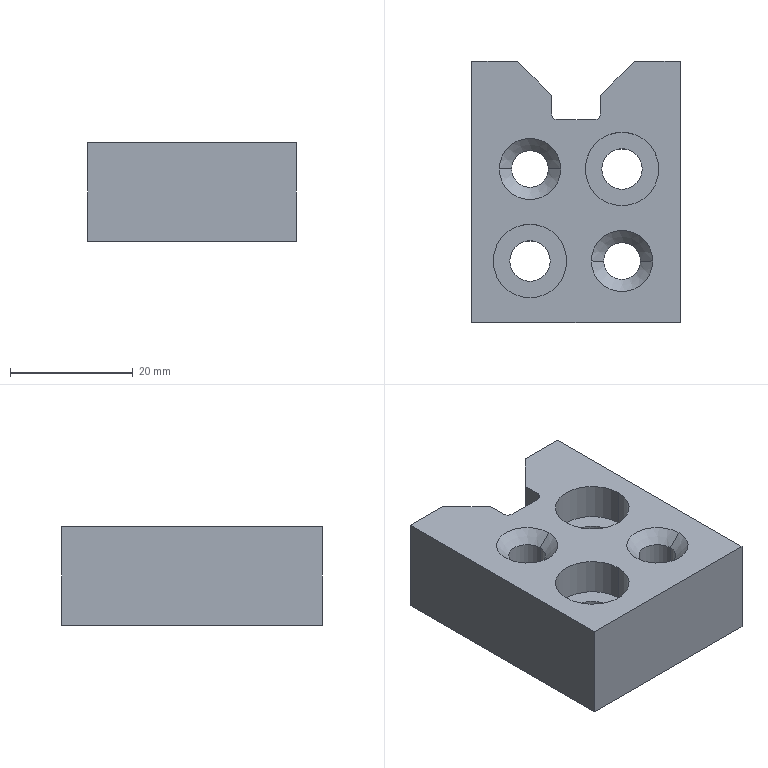Part | SolidWorks | features Chamfer 2, Cut 2, Fillet 2, HoleWzd 2, Extrusion 1, ICE 1 | 1 solid | 36 faces | box 34 x 42.517 x 16 mm | volume 18300 mm3 | cylinder 14 | plane 14 | cone 8 | commonest cylinder face diameters 6 x4 6.6 x4 12 x4 2 x2
STEP:
#1=CARTESIAN_POINT('',(-10.8,15.849,0.));
#2=VERTEX_POINT('',#1);
#3=CARTESIAN_POINT('',(-4.2,15.849,0.));
#4=VERTEX_POINT('',#3);
#5=CARTESIAN_POINT('',(-7.5,15.849,0.));
#6=DIRECTION('',(0.,0.,1.));
#7=DIRECTION('',(1.,0.,0.));
#8=AXIS2_PLACEMENT_3D('',#5,#6,#7);
#9=CIRCLE('',#8,3.3);
#10=EDGE_CURVE('',#2,#4,#9,.T.);
#11=ORIENTED_EDGE('',*,*,#10,.F.);
#12=CARTESIAN_POINT('',(-10.8,15.849,10.));
#13=VERTEX_POINT('',#12);
#14=CARTESIAN_POINT('',(-10.8,15.849,16.));
#15=DIRECTION('',(0.,0.,1.));
#16=VECTOR('',#15,1000.);
#17=LINE('',#14,#16);
#18=EDGE_CURVE('',#2,#13,#17,.T.);
#19=ORIENTED_EDGE('',*,*,#18,.T.);
#20=CARTESIAN_POINT('',(-4.2,15.849,10.));
#21=VERTEX_POINT('',#20);
#22=CARTESIAN_POINT('',(-7.5,15.849,10.));
#23=DIRECTION('',(0.,0.,1.));
#24=DIRECTION('',(1.,0.,0.));
#25=AXIS2_PLACEMENT_3D('',#22,#23,#24);
#26=CIRCLE('',#25,3.3);
#27=EDGE_CURVE('',#13,#21,#26,.T.);
#28=ORIENTED_EDGE('',*,*,#27,.T.);
#29=CARTESIAN_POINT('',(-4.2,15.849,16.));
#30=DIRECTION('',(0.,0.,1.));
#31=VECTOR('',#30,1000.);
#32=LINE('',#29,#31);
#33=EDGE_CURVE('',#4,#21,#32,.T.);
#34=ORIENTED_EDGE('',*,*,#33,.F.);
#35=EDGE_LOOP('',(#11,#19,#28,#34));
#36=FACE_OUTER_BOUND('',#35,.T.);
#37=CARTESIAN_POINT('',(-7.5,15.849,16.));
#38=DIRECTION('',(0.,0.,1.));
#39=DIRECTION('',(1.,0.,0.));
#40=AXIS2_PLACEMENT_3D('',#37,#38,#39);
#41=CYLINDRICAL_SURFACE('',#40,3.3);
#42=ADVANCED_FACE('',(#36),#41,.F.);
#43=CARTESIAN_POINT('',(-13.5,15.849,10.));
#44=VERTEX_POINT('',#43);
#45=CARTESIAN_POINT('',(-1.5,15.849,10.));
#46=VERTEX_POINT('',#45);
#47=CARTESIAN_POINT('',(-7.5,15.849,10.));
#48=DIRECTION('',(0.,0.,1.));
#49=DIRECTION('',(1.,0.,0.));
#50=AXIS2_PLACEMENT_3D('',#47,#48,#49);
#51=CIRCLE('',#50,6.);
#52=EDGE_CURVE('',#44,#46,#51,.T.);
#53=ORIENTED_EDGE('',*,*,#52,.F.);
#54=CARTESIAN_POINT('',(-13.5,15.849,16.));
#55=VERTEX_POINT('',#54);
#56=CARTESIAN_POINT('',(-13.5,15.849,16.));
#57=DIRECTION('',(0.,0.,1.));
#58=VECTOR('',#57,1000.);
#59=LINE('',#56,#58);
#60=EDGE_CURVE('',#44,#55,#59,.T.);
#61=ORIENTED_EDGE('',*,*,#60,.T.);
#62=CARTESIAN_POINT('',(-1.5,15.849,16.));
#63=VERTEX_POINT('',#62);
#64=CARTESIAN_POINT('',(-7.5,15.849,16.));
#65=DIRECTION('',(0.,0.,1.));
#66=DIRECTION('',(1.,0.,0.));
#67=AXIS2_PLACEMENT_3D('',#64,#65,#66);
#68=CIRCLE('',#67,6.);
#69=EDGE_CURVE('',#55,#63,#68,.T.);
#70=ORIENTED_EDGE('',*,*,#69,.T.);
#71=CARTESIAN_POINT('',(-1.5,15.849,16.));
#72=DIRECTION('',(0.,0.,1.));
#73=VECTOR('',#72,1000.);
#74=LINE('',#71,#73);
#75=EDGE_CURVE('',#46,#63,#74,.T.);
#76=ORIENTED_EDGE('',*,*,#75,.F.);
#77=EDGE_LOOP('',(#53,#61,#70,#76));
#78=FACE_OUTER_BOUND('',#77,.T.);
#79=CARTESIAN_POINT('',(-7.5,15.849,16.));
#80=DIRECTION('',(0.,0.,1.));
#81=DIRECTION('',(1.,0.,0.));
#82=AXIS2_PLACEMENT_3D('',#79,#80,#81);
#83=CYLINDRICAL_SURFACE('',#82,6.);
#84=ADVANCED_FACE('',(#78),#83,.F.);
#85=CARTESIAN_POINT('',(10.5,15.849,2.));
#86=VERTEX_POINT('',#85);
#87=CARTESIAN_POINT('',(4.5,15.849,2.));
#88=VERTEX_POINT('',#87);
#89=CARTESIAN_POINT('',(7.5,15.849,2.));
#90=DIRECTION('',(0.,0.,-1.));
#91=DIRECTION('',(1.,0.,0.));
#92=AXIS2_PLACEMENT_3D('',#89,#90,#91);
#93=CIRCLE('',#92,3.);
#94=EDGE_CURVE('',#86,#88,#93,.T.);
#95=ORIENTED_EDGE('',*,*,#94,.F.);
#96=CARTESIAN_POINT('',(12.5,15.849,0.));
#97=VERTEX_POINT('',#96);
#98=CARTESIAN_POINT('',(12.5,15.849,0.));
#99=DIRECTION('',(0.7071,0.,-0.7071));
#100=VECTOR('',#99,1000.);
#101=LINE('',#98,#100);
#102=EDGE_CURVE('',#86,#97,#101,.T.);
#103=ORIENTED_EDGE('',*,*,#102,.T.);
#104=CARTESIAN_POINT('',(2.5,15.849,0.));
#105=VERTEX_POINT('',#104);
#106=CARTESIAN_POINT('',(7.5,15.849,0.));
#107=DIRECTION('',(0.,0.,1.));
#108=DIRECTION('',(1.,0.,0.));
#109=AXIS2_PLACEMENT_3D('',#106,#107,#108);
#110=CIRCLE('',#109,5.);
#111=EDGE_CURVE('',#105,#97,#110,.T.);
#112=ORIENTED_EDGE('',*,*,#111,.F.);
#113=CARTESIAN_POINT('',(2.5,15.849,0.));
#114=DIRECTION('',(-0.7071,0.,-0.7071));
#115=VECTOR('',#114,1000.);
#116=LINE('',#113,#115);
#117=EDGE_CURVE('',#88,#105,#116,.T.);
#118=ORIENTED_EDGE('',*,*,#117,.F.);
#119=EDGE_LOOP('',(#95,#103,#112,#118));
#120=FACE_OUTER_BOUND('',#119,.T.);
#121=CARTESIAN_POINT('',(7.5,15.849,0.));
#122=DIRECTION('',(0.,0.,-1.));
#123=DIRECTION('',(-1.,0.,0.));
#124=AXIS2_PLACEMENT_3D('',#121,#122,#123);
#125=CONICAL_SURFACE('',#124,5.,0.7854);
#126=ADVANCED_FACE('',(#120),#125,.F.);
#127=CARTESIAN_POINT('',(-4.5,30.849,2.));
#128=VERTEX_POINT('',#127);
#129=CARTESIAN_POINT('',(-10.5,30.849,2.));
#130=VERTEX_POINT('',#129);
#131=CARTESIAN_POINT('',(-7.5,30.849,2.));
#132=DIRECTION('',(0.,0.,-1.));
#133=DIRECTION('',(1.,0.,0.));
#134=AXIS2_PLACEMENT_3D('',#131,#132,#133);
#135=CIRCLE('',#134,3.);
#136=EDGE_CURVE('',#128,#130,#135,.T.);
#137=ORIENTED_EDGE('',*,*,#136,.F.);
#138=CARTESIAN_POINT('',(-2.5,30.849,0.));
#139=VERTEX_POINT('',#138);
#140=CARTESIAN_POINT('',(-2.5,30.849,0.));
#141=DIRECTION('',(0.7071,0.,-0.7071));
#142=VECTOR('',#141,1000.);
#143=LINE('',#140,#142);
#144=EDGE_CURVE('',#128,#139,#143,.T.);
#145=ORIENTED_EDGE('',*,*,#144,.T.);
#146=CARTESIAN_POINT('',(-12.5,30.849,0.));
#147=VERTEX_POINT('',#146);
#148=CARTESIAN_POINT('',(-7.5,30.849,0.));
#149=DIRECTION('',(0.,0.,1.));
#150=DIRECTION('',(1.,0.,0.));
#151=AXIS2_PLACEMENT_3D('',#148,#149,#150);
#152=CIRCLE('',#151,5.);
#153=EDGE_CURVE('',#147,#139,#152,.T.);
#154=ORIENTED_EDGE('',*,*,#153,.F.);
#155=CARTESIAN_POINT('',(-12.5,30.849,0.));
#156=DIRECTION('',(-0.7071,0.,-0.7071));
#157=VECTOR('',#156,1000.);
#158=LINE('',#155,#157);
#159=EDGE_CURVE('',#130,#147,#158,.T.);
#160=ORIENTED_EDGE('',*,*,#159,.F.);
#161=EDGE_LOOP('',(#137,#145,#154,#160));
#162=FACE_OUTER_BOUND('',#161,.T.);
#163=CARTESIAN_POINT('',(-7.5,30.849,0.));
#164=DIRECTION('',(0.,0.,-1.));
#165=DIRECTION('',(-1.,0.,0.));
#166=AXIS2_PLACEMENT_3D('',#163,#164,#165);
#167=CONICAL_SURFACE('',#166,5.,0.7854);
#168=ADVANCED_FACE('',(#162),#167,.F.);
#169=CARTESIAN_POINT('',(4.5,15.849,14.));
#170=VERTEX_POINT('',#169);
#171=CARTESIAN_POINT('',(10.5,15.849,14.));
#172=VERTEX_POINT('',#171);
#173=CARTESIAN_POINT('',(7.5,15.849,14.));
#174=DIRECTION('',(0.,0.,1.));
#175=DIRECTION('',(1.,0.,0.));
#176=AXIS2_PLACEMENT_3D('',#173,#174,#175);
#177=CIRCLE('',#176,3.);
#178=EDGE_CURVE('',#170,#172,#177,.T.);
#179=ORIENTED_EDGE('',*,*,#178,.F.);
#180=CARTESIAN_POINT('',(2.5,15.849,16.));
#181=VERTEX_POINT('',#180);
#182=CARTESIAN_POINT('',(4.5,15.849,14.));
#183=DIRECTION('',(-0.7071,0.,0.7071));
#184=VECTOR('',#183,1000.);
#185=LINE('',#182,#184);
#186=EDGE_CURVE('',#170,#181,#185,.T.);
#187=ORIENTED_EDGE('',*,*,#186,.T.);
#188=CARTESIAN_POINT('',(12.5,15.849,16.));
#189=VERTEX_POINT('',#188);
#190=CARTESIAN_POINT('',(7.5,15.849,16.));
#191=DIRECTION('',(0.,0.,-1.));
#192=DIRECTION('',(1.,0.,0.));
#193=AXIS2_PLACEMENT_3D('',#190,#191,#192);
#194=CIRCLE('',#193,5.);
#195=EDGE_CURVE('',#189,#181,#194,.T.);
#196=ORIENTED_EDGE('',*,*,#195,.F.);
#197=CARTESIAN_POINT('',(10.5,15.849,14.));
#198=DIRECTION('',(0.7071,0.,0.7071));
#199=VECTOR('',#198,1000.);
#200=LINE('',#197,#199);
#201=EDGE_CURVE('',#172,#189,#200,.T.);
#202=ORIENTED_EDGE('',*,*,#201,.F.);
#203=EDGE_LOOP('',(#179,#187,#196,#202));
#204=FACE_OUTER_BOUND('',#203,.T.);
#205=CARTESIAN_POINT('',(7.5,15.849,14.));
#206=DIRECTION('',(0.,0.,1.));
#207=DIRECTION('',(1.,0.,0.));
#208=AXIS2_PLACEMENT_3D('',#205,#206,#207);
#209=CONICAL_SURFACE('',#208,3.,0.7854);
#210=ADVANCED_FACE('',(#204),#209,.F.);
#211=CARTESIAN_POINT('',(-10.5,30.849,14.));
#212=VERTEX_POINT('',#211);
#213=CARTESIAN_POINT('',(-4.5,30.849,14.));
#214=VERTEX_POINT('',#213);
#215=CARTESIAN_POINT('',(-7.5,30.849,14.));
#216=DIRECTION('',(0.,0.,1.));
#217=DIRECTION('',(1.,0.,0.));
#218=AXIS2_PLACEMENT_3D('',#215,#216,#217);
#219=CIRCLE('',#218,3.);
#220=EDGE_CURVE('',#212,#214,#219,.T.);
#221=ORIENTED_EDGE('',*,*,#220,.F.);
#222=CARTESIAN_POINT('',(-12.5,30.849,16.));
#223=VERTEX_POINT('',#222);
#224=CARTESIAN_POINT('',(-10.5,30.849,14.));
#225=DIRECTION('',(-0.7071,0.,0.7071));
#226=VECTOR('',#225,1000.);
#227=LINE('',#224,#226);
#228=EDGE_CURVE('',#212,#223,#227,.T.);
#229=ORIENTED_EDGE('',*,*,#228,.T.);
#230=CARTESIAN_POINT('',(-2.5,30.849,16.));
#231=VERTEX_POINT('',#230);
#232=CARTESIAN_POINT('',(-7.5,30.849,16.));
#233=DIRECTION('',(0.,0.,-1.));
#234=DIRECTION('',(1.,0.,0.));
#235=AXIS2_PLACEMENT_3D('',#232,#233,#234);
#236=CIRCLE('',#235,5.);
#237=EDGE_CURVE('',#231,#223,#236,.T.);
#238=ORIENTED_EDGE('',*,*,#237,.F.);
#239=CARTESIAN_POINT('',(-4.5,30.849,14.));
#240=DIRECTION('',(0.7071,0.,0.7071));
#241=VECTOR('',#240,1000.);
#242=LINE('',#239,#241);
#243=EDGE_CURVE('',#214,#231,#242,.T.);
#244=ORIENTED_EDGE('',*,*,#243,.F.);
#245=EDGE_LOOP('',(#221,#229,#238,#244));
#246=FACE_OUTER_BOUND('',#245,.T.);
#247=CARTESIAN_POINT('',(-7.5,30.849,14.));
#248=DIRECTION('',(0.,0.,1.));
#249=DIRECTION('',(1.,0.,0.));
#250=AXIS2_PLACEMENT_3D('',#247,#248,#249);
#251=CONICAL_SURFACE('',#250,3.,0.7854);
#252=ADVANCED_FACE('',(#246),#251,.F.);
#253=ORIENTED_EDGE('',*,*,#94,.T.);
#254=CARTESIAN_POINT('',(4.5,15.849,-9.));
#255=DIRECTION('',(0.,0.,1.));
#256=VECTOR('',#255,1000.);
#257=LINE('',#254,#256);
#258=EDGE_CURVE('',#88,#170,#257,.T.);
#259=ORIENTED_EDGE('',*,*,#258,.T.);
#260=ORIENTED_EDGE('',*,*,#178,.T.);
#261=CARTESIAN_POINT('',(10.5,15.849,-9.));
#262=DIRECTION('',(0.,0.,1.));
#263=VECTOR('',#262,1000.);
#264=LINE('',#261,#263);
#265=EDGE_CURVE('',#86,#172,#264,.T.);
#266=ORIENTED_EDGE('',*,*,#265,.F.);
#267=EDGE_LOOP('',(#253,#259,#260,#266));
#268=FACE_OUTER_BOUND('',#267,.T.);
#269=CARTESIAN_POINT('',(7.5,15.849,-9.));
#270=DIRECTION('',(0.,0.,1.));
#271=DIRECTION('',(1.,0.,0.));
#272=AXIS2_PLACEMENT_3D('',#269,#270,#271);
#273=CYLINDRICAL_SURFACE('',#272,3.);
#274=ADVANCED_FACE('',(#268),#273,.F.);
#275=ORIENTED_EDGE('',*,*,#136,.T.);
#276=CARTESIAN_POINT('',(-10.5,30.849,-9.));
#277=DIRECTION('',(0.,0.,1.));
#278=VECTOR('',#277,1000.);
#279=LINE('',#276,#278);
#280=EDGE_CURVE('',#130,#212,#279,.T.);
#281=ORIENTED_EDGE('',*,*,#280,.T.);
#282=ORIENTED_EDGE('',*,*,#220,.T.);
#283=CARTESIAN_POINT('',(-4.5,30.849,-9.));
#284=DIRECTION('',(0.,0.,1.));
#285=VECTOR('',#284,1000.);
#286=LINE('',#283,#285);
#287=EDGE_CURVE('',#128,#214,#286,.T.);
#288=ORIENTED_EDGE('',*,*,#287,.F.);
#289=EDGE_LOOP('',(#275,#281,#282,#288));
#290=FACE_OUTER_BOUND('',#289,.T.);
#291=CARTESIAN_POINT('',(-7.5,30.849,-9.));
#292=DIRECTION('',(0.,0.,1.));
#293=DIRECTION('',(1.,0.,0.));
#294=AXIS2_PLACEMENT_3D('',#291,#292,#293);
#295=CYLINDRICAL_SURFACE('',#294,3.);
#296=ADVANCED_FACE('',(#290),#295,.F.);
#297=CARTESIAN_POINT('',(4.2,30.849,0.));
#298=VERTEX_POINT('',#297);
#299=CARTESIAN_POINT('',(10.8,30.849,0.));
#300=VERTEX_POINT('',#299);
#301=CARTESIAN_POINT('',(7.5,30.849,0.));
#302=DIRECTION('',(0.,0.,1.));
#303=DIRECTION('',(1.,0.,0.));
#304=AXIS2_PLACEMENT_3D('',#301,#302,#303);
#305=CIRCLE('',#304,3.3);
#306=EDGE_CURVE('',#298,#300,#305,.T.);
#307=ORIENTED_EDGE('',*,*,#306,.F.);
#308=CARTESIAN_POINT('',(4.2,30.849,10.));
#309=VERTEX_POINT('',#308);
#310=CARTESIAN_POINT('',(4.2,30.849,16.));
#311=DIRECTION('',(0.,0.,1.));
#312=VECTOR('',#311,1000.);
#313=LINE('',#310,#312);
#314=EDGE_CURVE('',#298,#309,#313,.T.);
#315=ORIENTED_EDGE('',*,*,#314,.T.);
#316=CARTESIAN_POINT('',(10.8,30.849,10.));
#317=VERTEX_POINT('',#316);
#318=CARTESIAN_POINT('',(7.5,30.849,10.));
#319=DIRECTION('',(0.,0.,1.));
#320=DIRECTION('',(1.,0.,0.));
#321=AXIS2_PLACEMENT_3D('',#318,#319,#320);
#322=CIRCLE('',#321,3.3);
#323=EDGE_CURVE('',#309,#317,#322,.T.);
#324=ORIENTED_EDGE('',*,*,#323,.T.);
#325=CARTESIAN_POINT('',(10.8,30.849,16.));
#326=DIRECTION('',(0.,0.,1.));
#327=VECTOR('',#326,1000.);
#328=LINE('',#325,#327);
#329=EDGE_CURVE('',#300,#317,#328,.T.);
#330=ORIENTED_EDGE('',*,*,#329,.F.);
#331=EDGE_LOOP('',(#307,#315,#324,#330));
#332=FACE_OUTER_BOUND('',#331,.T.);
#333=CARTESIAN_POINT('',(7.5,30.849,16.));
#334=DIRECTION('',(0.,0.,1.));
#335=DIRECTION('',(1.,0.,0.));
#336=AXIS2_PLACEMENT_3D('',#333,#334,#335);
#337=CYLINDRICAL_SURFACE('',#336,3.3);
#338=ADVANCED_FACE('',(#332),#337,.F.);
#339=CARTESIAN_POINT('',(1.5,30.849,10.));
#340=VERTEX_POINT('',#339);
#341=CARTESIAN_POINT('',(13.5,30.849,10.));
#342=VERTEX_POINT('',#341);
#343=CARTESIAN_POINT('',(7.5,30.849,10.));
#344=DIRECTION('',(0.,0.,1.));
#345=DIRECTION('',(1.,0.,0.));
#346=AXIS2_PLACEMENT_3D('',#343,#344,#345);
#347=CIRCLE('',#346,6.);
#348=EDGE_CURVE('',#340,#342,#347,.T.);
#349=ORIENTED_EDGE('',*,*,#348,.F.);
#350=CARTESIAN_POINT('',(1.5,30.849,16.));
#351=VERTEX_POINT('',#350);
#352=CARTESIAN_POINT('',(1.5,30.849,16.));
#353=DIRECTION('',(0.,0.,1.));
#354=VECTOR('',#353,1000.);
#355=LINE('',#352,#354);
#356=EDGE_CURVE('',#340,#351,#355,.T.);
#357=ORIENTED_EDGE('',*,*,#356,.T.);
#358=CARTESIAN_POINT('',(13.5,30.849,16.));
#359=VERTEX_POINT('',#358);
#360=CARTESIAN_POINT('',(7.5,30.849,16.));
#361=DIRECTION('',(0.,0.,1.));
#362=DIRECTION('',(1.,0.,0.));
#363=AXIS2_PLACEMENT_3D('',#360,#361,#362);
#364=CIRCLE('',#363,6.);
#365=EDGE_CURVE('',#351,#359,#364,.T.);
#366=ORIENTED_EDGE('',*,*,#365,.T.);
#367=CARTESIAN_POINT('',(13.5,30.849,16.));
#368=DIRECTION('',(0.,0.,1.));
#369=VECTOR('',#368,1000.);
#370=LINE('',#367,#369);
#371=EDGE_CURVE('',#342,#359,#370,.T.);
#372=ORIENTED_EDGE('',*,*,#371,.F.);
#373=EDGE_LOOP('',(#349,#357,#366,#372));
#374=FACE_OUTER_BOUND('',#373,.T.);
#375=CARTESIAN_POINT('',(7.5,30.849,16.));
#376=DIRECTION('',(0.,0.,1.));
#377=DIRECTION('',(1.,0.,0.));
#378=AXIS2_PLACEMENT_3D('',#375,#376,#377);
#379=CYLINDRICAL_SURFACE('',#378,6.);
#380=ADVANCED_FACE('',(#374),#379,.F.);
#381=CARTESIAN_POINT('',(-17.,48.365,16.));
#382=VERTEX_POINT('',#381);
#383=CARTESIAN_POINT('',(-17.,5.849,16.));
#384=VERTEX_POINT('',#383);
#385=CARTESIAN_POINT('',(-17.,50.849,16.));
#386=DIRECTION('',(0.,-1.,0.));
#387=VECTOR('',#386,1000.);
#388=LINE('',#385,#387);
#389=EDGE_CURVE('',#382,#384,#388,.T.);
#390=ORIENTED_EDGE('',*,*,#389,.F.);
#391=CARTESIAN_POINT('',(-17.,48.365,0.));
#392=VERTEX_POINT('',#391);
#393=CARTESIAN_POINT('',(-17.,48.365,16.));
#394=DIRECTION('',(0.,0.,-1.));
#395=VECTOR('',#394,1000.);
#396=LINE('',#393,#395);
#397=EDGE_CURVE('',#382,#392,#396,.T.);
#398=ORIENTED_EDGE('',*,*,#397,.T.);
#399=CARTESIAN_POINT('',(-17.,5.849,0.));
#400=VERTEX_POINT('',#399);
#401=CARTESIAN_POINT('',(-17.,50.849,0.));
#402=DIRECTION('',(0.,-1.,0.));
#403=VECTOR('',#402,1000.);
#404=LINE('',#401,#403);
#405=EDGE_CURVE('',#392,#400,#404,.T.);
#406=ORIENTED_EDGE('',*,*,#405,.T.);
#407=CARTESIAN_POINT('',(-17.,5.849,16.));
#408=DIRECTION('',(0.,0.,-1.));
#409=VECTOR('',#408,1000.);
#410=LINE('',#407,#409);
#411=EDGE_CURVE('',#384,#400,#410,.T.);
#412=ORIENTED_EDGE('',*,*,#411,.F.);
#413=EDGE_LOOP('',(#390,#398,#406,#412));
#414=FACE_OUTER_BOUND('',#413,.T.);
#415=CARTESIAN_POINT('',(-17.,50.849,16.));
#416=DIRECTION('',(1.,0.,0.));
#417=DIRECTION('',(0.,1.,0.));
#418=AXIS2_PLACEMENT_3D('',#415,#416,#417);
#419=PLANE('',#418);
#420=ADVANCED_FACE('',(#414),#419,.F.);
#421=CARTESIAN_POINT('',(17.,5.849,0.));
#422=VERTEX_POINT('',#421);
#423=CARTESIAN_POINT('',(-17.,5.849,0.));
#424=DIRECTION('',(1.,0.,0.));
#425=VECTOR('',#424,1000.);
#426=LINE('',#423,#425);
#427=EDGE_CURVE('',#400,#422,#426,.T.);
#428=ORIENTED_EDGE('',*,*,#427,.T.);
#429=CARTESIAN_POINT('',(17.,5.849,16.));
#430=VERTEX_POINT('',#429);
#431=CARTESIAN_POINT('',(17.,5.849,16.));
#432=DIRECTION('',(0.,0.,-1.));
#433=VECTOR('',#432,1000.);
#434=LINE('',#431,#433);
#435=EDGE_CURVE('',#430,#422,#434,.T.);
#436=ORIENTED_EDGE('',*,*,#435,.F.);
#437=CARTESIAN_POINT('',(-17.,5.849,16.));
#438=DIRECTION('',(1.,0.,0.));
#439=VECTOR('',#438,1000.);
#440=LINE('',#437,#439);
#441=EDGE_CURVE('',#384,#430,#440,.T.);
#442=ORIENTED_EDGE('',*,*,#441,.F.);
#443=ORIENTED_EDGE('',*,*,#411,.T.);
#444=EDGE_LOOP('',(#428,#436,#442,#443));
#445=FACE_OUTER_BOUND('',#444,.T.);
#446=CARTESIAN_POINT('',(-17.,5.849,16.));
#447=DIRECTION('',(0.,1.,0.));
#448=DIRECTION('',(-1.,0.,0.));
#449=AXIS2_PLACEMENT_3D('',#446,#447,#448);
#450=PLANE('',#449);
#451=ADVANCED_FACE('',(#445),#450,.F.);
#452=CARTESIAN_POINT('',(17.,48.365,0.));
#453=VERTEX_POINT('',#452);
#454=CARTESIAN_POINT('',(17.,50.849,0.));
#455=DIRECTION('',(0.,1.,0.));
#456=VECTOR('',#455,1000.);
#457=LINE('',#454,#456);
#458=EDGE_CURVE('',#422,#453,#457,.T.);
#459=ORIENTED_EDGE('',*,*,#458,.T.);
#460=CARTESIAN_POINT('',(17.,48.365,16.));
#461=VERTEX_POINT('',#460);
#462=CARTESIAN_POINT('',(17.,48.365,16.));
#463=DIRECTION('',(0.,0.,1.));
#464=VECTOR('',#463,1000.);
#465=LINE('',#462,#464);
#466=EDGE_CURVE('',#453,#461,#465,.T.);
#467=ORIENTED_EDGE('',*,*,#466,.T.);
#468=CARTESIAN_POINT('',(17.,50.849,16.));
#469=DIRECTION('',(0.,1.,0.));
#470=VECTOR('',#469,1000.);
#471=LINE('',#468,#470);
#472=EDGE_CURVE('',#430,#461,#471,.T.);
#473=ORIENTED_EDGE('',*,*,#472,.F.);
#474=ORIENTED_EDGE('',*,*,#435,.T.);
#475=EDGE_LOOP('',(#459,#467,#473,#474));
#476=FACE_OUTER_BOUND('',#475,.T.);
#477=CARTESIAN_POINT('',(17.,50.849,16.));
#478=DIRECTION('',(-1.,0.,0.));
#479=DIRECTION('',(0.,-1.,0.));
#480=AXIS2_PLACEMENT_3D('',#477,#478,#479);
#481=PLANE('',#480);
#482=ADVANCED_FACE('',(#476),#481,.F.);
#483=CARTESIAN_POINT('',(-9.517,48.365,16.));
#484=VERTEX_POINT('',#483);
#485=CARTESIAN_POINT('',(-19.125,48.365,16.));
#486=DIRECTION('',(1.,0.,0.));
#487=VECTOR('',#486,1000.);
#488=LINE('',#485,#487);
#489=EDGE_CURVE('',#382,#484,#488,.T.);
#490=ORIENTED_EDGE('',*,*,#489,.F.);
#491=ORIENTED_EDGE('',*,*,#389,.T.);
#492=ORIENTED_EDGE('',*,*,#441,.T.);
#493=ORIENTED_EDGE('',*,*,#472,.T.);
#494=CARTESIAN_POINT('',(9.517,48.365,16.));
#495=VERTEX_POINT('',#494);
#496=CARTESIAN_POINT('',(-19.125,48.365,16.));
#497=DIRECTION('',(1.,0.,0.));
#498=VECTOR('',#497,1000.);
#499=LINE('',#496,#498);
#500=EDGE_CURVE('',#495,#461,#499,.T.);
#501=ORIENTED_EDGE('',*,*,#500,.F.);
#502=CARTESIAN_POINT('',(4.,42.849,16.));
#503=VERTEX_POINT('',#502);
#504=CARTESIAN_POINT('',(12.,50.849,16.));
#505=DIRECTION('',(0.7071,0.7071,0.));
#506=VECTOR('',#505,1000.);
#507=LINE('',#504,#506);
#508=EDGE_CURVE('',#503,#495,#507,.T.);
#509=ORIENTED_EDGE('',*,*,#508,.F.);
#510=CARTESIAN_POINT('',(4.,39.849,16.));
#511=VERTEX_POINT('',#510);
#512=CARTESIAN_POINT('',(4.,38.849,16.));
#513=DIRECTION('',(0.,1.,0.));
#514=VECTOR('',#513,1000.);
#515=LINE('',#512,#514);
#516=EDGE_CURVE('',#511,#503,#515,.T.);
#517=ORIENTED_EDGE('',*,*,#516,.F.);
#518=CARTESIAN_POINT('',(3.,38.849,16.));
#519=VERTEX_POINT('',#518);
#520=CARTESIAN_POINT('',(3.,39.849,16.));
#521=DIRECTION('',(0.,0.,-1.));
#522=DIRECTION('',(1.,0.,0.));
#523=AXIS2_PLACEMENT_3D('',#520,#521,#522);
#524=CIRCLE('',#523,1.);
#525=EDGE_CURVE('',#511,#519,#524,.T.);
#526=ORIENTED_EDGE('',*,*,#525,.T.);
#527=CARTESIAN_POINT('',(-3.,38.849,16.));
#528=VERTEX_POINT('',#527);
#529=CARTESIAN_POINT('',(-4.,38.849,16.));
#530=DIRECTION('',(1.,0.,0.));
#531=VECTOR('',#530,1000.);
#532=LINE('',#529,#531);
#533=EDGE_CURVE('',#528,#519,#532,.T.);
#534=ORIENTED_EDGE('',*,*,#533,.F.);
#535=CARTESIAN_POINT('',(-4.,39.849,16.));
#536=VERTEX_POINT('',#535);
#537=CARTESIAN_POINT('',(-3.,39.849,16.));
#538=DIRECTION('',(0.,0.,-1.));
#539=DIRECTION('',(1.,0.,0.));
#540=AXIS2_PLACEMENT_3D('',#537,#538,#539);
#541=CIRCLE('',#540,1.);
#542=EDGE_CURVE('',#528,#536,#541,.T.);
#543=ORIENTED_EDGE('',*,*,#542,.T.);
#544=CARTESIAN_POINT('',(-4.,42.849,16.));
#545=VERTEX_POINT('',#544);
#546=CARTESIAN_POINT('',(-4.,38.849,16.));
#547=DIRECTION('',(0.,-1.,0.));
#548=VECTOR('',#547,1000.);
#549=LINE('',#546,#548);
#550=EDGE_CURVE('',#545,#536,#549,.T.);
#551=ORIENTED_EDGE('',*,*,#550,.F.);
#552=CARTESIAN_POINT('',(-12.,50.849,16.));
#553=DIRECTION('',(0.7071,-0.7071,0.));
#554=VECTOR('',#553,1000.);
#555=LINE('',#552,#554);
#556=EDGE_CURVE('',#484,#545,#555,.T.);
#557=ORIENTED_EDGE('',*,*,#556,.F.);
#558=EDGE_LOOP('',(#490,#491,#492,#493,#501,#509,#517,#526,#534,#543,#551,#557));
#559=FACE_OUTER_BOUND('',#558,.T.);
#560=CARTESIAN_POINT('',(-7.5,15.849,16.));
#561=DIRECTION('',(0.,0.,1.));
#562=DIRECTION('',(1.,0.,0.));
#563=AXIS2_PLACEMENT_3D('',#560,#561,#562);
#564=CIRCLE('',#563,6.);
#565=EDGE_CURVE('',#63,#55,#564,.T.);
#566=ORIENTED_EDGE('',*,*,#565,.F.);
#567=ORIENTED_EDGE('',*,*,#69,.F.);
#568=EDGE_LOOP('',(#566,#567));
#569=FACE_BOUND('',#568,.T.);
#570=ORIENTED_EDGE('',*,*,#237,.T.);
#571=CARTESIAN_POINT('',(-7.5,30.849,16.));
#572=DIRECTION('',(0.,0.,-1.));
#573=DIRECTION('',(1.,0.,0.));
#574=AXIS2_PLACEMENT_3D('',#571,#572,#573);
#575=CIRCLE('',#574,5.);
#576=EDGE_CURVE('',#223,#231,#575,.T.);
#577=ORIENTED_EDGE('',*,*,#576,.T.);
#578=EDGE_LOOP('',(#570,#577));
#579=FACE_BOUND('',#578,.T.);
#580=ORIENTED_EDGE('',*,*,#195,.T.);
#581=CARTESIAN_POINT('',(7.5,15.849,16.));
#582=DIRECTION('',(0.,0.,-1.));
#583=DIRECTION('',(1.,0.,0.));
#584=AXIS2_PLACEMENT_3D('',#581,#582,#583);
#585=CIRCLE('',#584,5.);
#586=EDGE_CURVE('',#181,#189,#585,.T.);
#587=ORIENTED_EDGE('',*,*,#586,.T.);
#588=EDGE_LOOP('',(#580,#587));
#589=FACE_BOUND('',#588,.T.);
#590=CARTESIAN_POINT('',(7.5,30.849,16.));
#591=DIRECTION('',(0.,0.,1.));
#592=DIRECTION('',(1.,0.,0.));
#593=AXIS2_PLACEMENT_3D('',#590,#591,#592);
#594=CIRCLE('',#593,6.);
#595=EDGE_CURVE('',#359,#351,#594,.T.);
#596=ORIENTED_EDGE('',*,*,#595,.F.);
#597=ORIENTED_EDGE('',*,*,#365,.F.);
#598=EDGE_LOOP('',(#596,#597));
#599=FACE_BOUND('',#598,.T.);
#600=CARTESIAN_POINT('',(-17.,5.849,16.));
#601=DIRECTION('',(0.,0.,1.));
#602=DIRECTION('',(1.,0.,0.));
#603=AXIS2_PLACEMENT_3D('',#600,#601,#602);
#604=PLANE('',#603);
#605=ADVANCED_FACE('',(#559,#569,#579,#589,#599),#604,.T.);
#606=CARTESIAN_POINT('',(-7.5,15.849,0.));
#607=DIRECTION('',(0.,0.,1.));
#608=DIRECTION('',(1.,0.,0.));
#609=AXIS2_PLACEMENT_3D('',#606,#607,#608);
#610=CIRCLE('',#609,3.3);
#611=EDGE_CURVE('',#4,#2,#610,.T.);
#612=ORIENTED_EDGE('',*,*,#611,.T.);
#613=ORIENTED_EDGE('',*,*,#10,.T.);
#614=EDGE_LOOP('',(#612,#613));
#615=FACE_BOUND('',#614,.T.);
#616=ORIENTED_EDGE('',*,*,#153,.T.);
#617=CARTESIAN_POINT('',(-7.5,30.849,0.));
#618=DIRECTION('',(0.,0.,1.));
#619=DIRECTION('',(1.,0.,0.));
#620=AXIS2_PLACEMENT_3D('',#617,#618,#619);
#621=CIRCLE('',#620,5.);
#622=EDGE_CURVE('',#139,#147,#621,.T.);
#623=ORIENTED_EDGE('',*,*,#622,.T.);
#624=EDGE_LOOP('',(#616,#623));
#625=FACE_BOUND('',#624,.T.);
#626=ORIENTED_EDGE('',*,*,#111,.T.);
#627=CARTESIAN_POINT('',(7.5,15.849,0.));
#628=DIRECTION('',(0.,0.,1.));
#629=DIRECTION('',(1.,0.,0.));
#630=AXIS2_PLACEMENT_3D('',#627,#628,#629);
#631=CIRCLE('',#630,5.);
#632=EDGE_CURVE('',#97,#105,#631,.T.);
#633=ORIENTED_EDGE('',*,*,#632,.T.);
#634=EDGE_LOOP('',(#626,#633));
#635=FACE_BOUND('',#634,.T.);
#636=CARTESIAN_POINT('',(7.5,30.849,0.));
#637=DIRECTION('',(0.,0.,1.));
#638=DIRECTION('',(1.,0.,0.));
#639=AXIS2_PLACEMENT_3D('',#636,#637,#638);
#640=CIRCLE('',#639,3.3);
#641=EDGE_CURVE('',#300,#298,#640,.T.);
#642=ORIENTED_EDGE('',*,*,#641,.T.);
#643=ORIENTED_EDGE('',*,*,#306,.T.);
#644=EDGE_LOOP('',(#642,#643));
#645=FACE_BOUND('',#644,.T.);
#646=ORIENTED_EDGE('',*,*,#405,.F.);
#647=CARTESIAN_POINT('',(-9.517,48.365,0.));
#648=VERTEX_POINT('',#647);
#649=CARTESIAN_POINT('',(-19.125,48.365,0.));
#650=DIRECTION('',(1.,0.,0.));
#651=VECTOR('',#650,1000.);
#652=LINE('',#649,#651);
#653=EDGE_CURVE('',#392,#648,#652,.T.);
#654=ORIENTED_EDGE('',*,*,#653,.T.);
#655=CARTESIAN_POINT('',(-4.,42.849,0.));
#656=VERTEX_POINT('',#655);
#657=CARTESIAN_POINT('',(-12.,50.849,0.));
#658=DIRECTION('',(0.7071,-0.7071,0.));
#659=VECTOR('',#658,1000.);
#660=LINE('',#657,#659);
#661=EDGE_CURVE('',#648,#656,#660,.T.);
#662=ORIENTED_EDGE('',*,*,#661,.T.);
#663=CARTESIAN_POINT('',(-4.,39.849,0.));
#664=VERTEX_POINT('',#663);
#665=CARTESIAN_POINT('',(-4.,38.849,0.));
#666=DIRECTION('',(0.,-1.,0.));
#667=VECTOR('',#666,1000.);
#668=LINE('',#665,#667);
#669=EDGE_CURVE('',#656,#664,#668,.T.);
#670=ORIENTED_EDGE('',*,*,#669,.T.);
#671=CARTESIAN_POINT('',(-3.,38.849,0.));
#672=VERTEX_POINT('',#671);
#673=CARTESIAN_POINT('',(-3.,39.849,0.));
#674=DIRECTION('',(0.,0.,1.));
#675=DIRECTION('',(1.,0.,0.));
#676=AXIS2_PLACEMENT_3D('',#673,#674,#675);
#677=CIRCLE('',#676,1.);
#678=EDGE_CURVE('',#664,#672,#677,.T.);
#679=ORIENTED_EDGE('',*,*,#678,.T.);
#680=CARTESIAN_POINT('',(3.,38.849,0.));
#681=VERTEX_POINT('',#680);
#682=CARTESIAN_POINT('',(-4.,38.849,0.));
#683=DIRECTION('',(1.,0.,0.));
#684=VECTOR('',#683,1000.);
#685=LINE('',#682,#684);
#686=EDGE_CURVE('',#672,#681,#685,.T.);
#687=ORIENTED_EDGE('',*,*,#686,.T.);
#688=CARTESIAN_POINT('',(4.,39.849,0.));
#689=VERTEX_POINT('',#688);
#690=CARTESIAN_POINT('',(3.,39.849,0.));
#691=DIRECTION('',(0.,0.,1.));
#692=DIRECTION('',(1.,0.,0.));
#693=AXIS2_PLACEMENT_3D('',#690,#691,#692);
#694=CIRCLE('',#693,1.);
#695=EDGE_CURVE('',#681,#689,#694,.T.);
#696=ORIENTED_EDGE('',*,*,#695,.T.);
#697=CARTESIAN_POINT('',(4.,42.849,0.));
#698=VERTEX_POINT('',#697);
#699=CARTESIAN_POINT('',(4.,38.849,0.));
#700=DIRECTION('',(0.,1.,0.));
#701=VECTOR('',#700,1000.);
#702=LINE('',#699,#701);
#703=EDGE_CURVE('',#689,#698,#702,.T.);
#704=ORIENTED_EDGE('',*,*,#703,.T.);
#705=CARTESIAN_POINT('',(9.517,48.365,0.));
#706=VERTEX_POINT('',#705);
#707=CARTESIAN_POINT('',(12.,50.849,0.));
#708=DIRECTION('',(0.7071,0.7071,0.));
#709=VECTOR('',#708,1000.);
#710=LINE('',#707,#709);
#711=EDGE_CURVE('',#698,#706,#710,.T.);
#712=ORIENTED_EDGE('',*,*,#711,.T.);
#713=CARTESIAN_POINT('',(-19.125,48.365,0.));
#714=DIRECTION('',(1.,0.,0.));
#715=VECTOR('',#714,1000.);
#716=LINE('',#713,#715);
#717=EDGE_CURVE('',#706,#453,#716,.T.);
#718=ORIENTED_EDGE('',*,*,#717,.T.);
#719=ORIENTED_EDGE('',*,*,#458,.F.);
#720=ORIENTED_EDGE('',*,*,#427,.F.);
#721=EDGE_LOOP('',(#646,#654,#662,#670,#679,#687,#696,#704,#712,#718,#719,#720));
#722=FACE_OUTER_BOUND('',#721,.T.);
#723=CARTESIAN_POINT('',(-17.,5.849,0.));
#724=DIRECTION('',(0.,0.,1.));
#725=DIRECTION('',(1.,0.,0.));
#726=AXIS2_PLACEMENT_3D('',#723,#724,#725);
#727=PLANE('',#726);
#728=ADVANCED_FACE('',(#615,#625,#635,#645,#722),#727,.F.);
#729=ORIENTED_EDGE('',*,*,#550,.T.);
#730=CARTESIAN_POINT('',(-4.,39.849,0.));
#731=DIRECTION('',(0.,0.,-1.));
#732=VECTOR('',#731,1000.);
#733=LINE('',#730,#732);
#734=EDGE_CURVE('',#536,#664,#733,.T.);
#735=ORIENTED_EDGE('',*,*,#734,.T.);
#736=ORIENTED_EDGE('',*,*,#669,.F.);
#737=CARTESIAN_POINT('',(-4.,42.849,0.));
#738=DIRECTION('',(0.,0.,1.));
#739=VECTOR('',#738,1000.);
#740=LINE('',#737,#739);
#741=EDGE_CURVE('',#656,#545,#740,.T.);
#742=ORIENTED_EDGE('',*,*,#741,.T.);
#743=EDGE_LOOP('',(#729,#735,#736,#742));
#744=FACE_OUTER_BOUND('',#743,.T.);
#745=CARTESIAN_POINT('',(-4.,38.849,0.));
#746=DIRECTION('',(-1.,0.,0.));
#747=DIRECTION('',(0.,-1.,0.));
#748=AXIS2_PLACEMENT_3D('',#745,#746,#747);
#749=PLANE('',#748);
#750=ADVANCED_FACE('',(#744),#749,.F.);
#751=ORIENTED_EDGE('',*,*,#661,.F.);
#752=CARTESIAN_POINT('',(-9.517,48.365,0.));
#753=DIRECTION('',(0.,0.,1.));
#754=VECTOR('',#753,1000.);
#755=LINE('',#752,#754);
#756=EDGE_CURVE('',#648,#484,#755,.T.);
#757=ORIENTED_EDGE('',*,*,#756,.T.);
#758=ORIENTED_EDGE('',*,*,#556,.T.);
#759=ORIENTED_EDGE('',*,*,#741,.F.);
#760=EDGE_LOOP('',(#751,#757,#758,#759));
#761=FACE_OUTER_BOUND('',#760,.T.);
#762=CARTESIAN_POINT('',(-12.,50.849,0.));
#763=DIRECTION('',(-0.7071,-0.7071,0.));
#764=DIRECTION('',(0.7071,-0.7071,0.));
#765=AXIS2_PLACEMENT_3D('',#762,#763,#764);
#766=PLANE('',#765);
#767=ADVANCED_FACE('',(#761),#766,.F.);
#768=ORIENTED_EDGE('',*,*,#508,.T.);
#769=CARTESIAN_POINT('',(9.517,48.365,0.));
#770=DIRECTION('',(0.,0.,-1.));
#771=VECTOR('',#770,1000.);
#772=LINE('',#769,#771);
#773=EDGE_CURVE('',#495,#706,#772,.T.);
#774=ORIENTED_EDGE('',*,*,#773,.T.);
#775=ORIENTED_EDGE('',*,*,#711,.F.);
#776=CARTESIAN_POINT('',(4.,42.849,0.));
#777=DIRECTION('',(0.,0.,1.));
#778=VECTOR('',#777,1000.);
#779=LINE('',#776,#778);
#780=EDGE_CURVE('',#698,#503,#779,.T.);
#781=ORIENTED_EDGE('',*,*,#780,.T.);
#782=EDGE_LOOP('',(#768,#774,#775,#781));
#783=FACE_OUTER_BOUND('',#782,.T.);
#784=CARTESIAN_POINT('',(12.,50.849,0.));
#785=DIRECTION('',(0.7071,-0.7071,0.));
#786=DIRECTION('',(0.7071,0.7071,0.));
#787=AXIS2_PLACEMENT_3D('',#784,#785,#786);
#788=PLANE('',#787);
#789=ADVANCED_FACE('',(#783),#788,.F.);
#790=ORIENTED_EDGE('',*,*,#703,.F.);
#791=CARTESIAN_POINT('',(4.,39.849,16.));
#792=DIRECTION('',(0.,0.,1.));
#793=VECTOR('',#792,1000.);
#794=LINE('',#791,#793);
#795=EDGE_CURVE('',#689,#511,#794,.T.);
#796=ORIENTED_EDGE('',*,*,#795,.T.);
#797=ORIENTED_EDGE('',*,*,#516,.T.);
#798=ORIENTED_EDGE('',*,*,#780,.F.);
#799=EDGE_LOOP('',(#790,#796,#797,#798));
#800=FACE_OUTER_BOUND('',#799,.T.);
#801=CARTESIAN_POINT('',(4.,38.849,0.));
#802=DIRECTION('',(1.,0.,0.));
#803=DIRECTION('',(0.,0.,-1.));
#804=AXIS2_PLACEMENT_3D('',#801,#802,#803);
#805=PLANE('',#804);
#806=ADVANCED_FACE('',(#800),#805,.F.);
#807=ORIENTED_EDGE('',*,*,#533,.T.);
#808=CARTESIAN_POINT('',(3.,38.849,0.));
#809=DIRECTION('',(0.,0.,-1.));
#810=VECTOR('',#809,1000.);
#811=LINE('',#808,#810);
#812=EDGE_CURVE('',#519,#681,#811,.T.);
#813=ORIENTED_EDGE('',*,*,#812,.T.);
#814=ORIENTED_EDGE('',*,*,#686,.F.);
#815=CARTESIAN_POINT('',(-3.,38.849,16.));
#816=DIRECTION('',(0.,0.,1.));
#817=VECTOR('',#816,1000.);
#818=LINE('',#815,#817);
#819=EDGE_CURVE('',#672,#528,#818,.T.);
#820=ORIENTED_EDGE('',*,*,#819,.T.);
#821=EDGE_LOOP('',(#807,#813,#814,#820));
#822=FACE_OUTER_BOUND('',#821,.T.);
#823=CARTESIAN_POINT('',(-4.,38.849,0.));
#824=DIRECTION('',(0.,-1.,0.));
#825=DIRECTION('',(1.,0.,0.));
#826=AXIS2_PLACEMENT_3D('',#823,#824,#825);
#827=PLANE('',#826);
#828=ADVANCED_FACE('',(#822),#827,.F.);
#829=ORIENTED_EDGE('',*,*,#356,.F.);
#830=CARTESIAN_POINT('',(7.5,30.849,10.));
#831=DIRECTION('',(0.,0.,1.));
#832=DIRECTION('',(1.,0.,0.));
#833=AXIS2_PLACEMENT_3D('',#830,#831,#832);
#834=CIRCLE('',#833,6.);
#835=EDGE_CURVE('',#342,#340,#834,.T.);
#836=ORIENTED_EDGE('',*,*,#835,.F.);
#837=ORIENTED_EDGE('',*,*,#371,.T.);
#838=ORIENTED_EDGE('',*,*,#595,.T.);
#839=EDGE_LOOP('',(#829,#836,#837,#838));
#840=FACE_OUTER_BOUND('',#839,.T.);
#841=CARTESIAN_POINT('',(7.5,30.849,16.));
#842=DIRECTION('',(0.,0.,1.));
#843=DIRECTION('',(1.,0.,0.));
#844=AXIS2_PLACEMENT_3D('',#841,#842,#843);
#845=CYLINDRICAL_SURFACE('',#844,6.);
#846=ADVANCED_FACE('',(#840),#845,.F.);
#847=CARTESIAN_POINT('',(7.5,30.849,10.));
#848=DIRECTION('',(0.,0.,1.));
#849=DIRECTION('',(1.,0.,0.));
#850=AXIS2_PLACEMENT_3D('',#847,#848,#849);
#851=CIRCLE('',#850,3.3);
#852=EDGE_CURVE('',#317,#309,#851,.T.);
#853=ORIENTED_EDGE('',*,*,#852,.F.);
#854=ORIENTED_EDGE('',*,*,#323,.F.);
#855=EDGE_LOOP('',(#853,#854));
#856=FACE_BOUND('',#855,.T.);
#857=ORIENTED_EDGE('',*,*,#835,.T.);
#858=ORIENTED_EDGE('',*,*,#348,.T.);
#859=EDGE_LOOP('',(#857,#858));
#860=FACE_OUTER_BOUND('',#859,.T.);
#861=CARTESIAN_POINT('',(10.8,30.849,10.));
#862=DIRECTION('',(0.,0.,-1.));
#863=DIRECTION('',(-1.,0.,0.));
#864=AXIS2_PLACEMENT_3D('',#861,#862,#863);
#865=PLANE('',#864);
#866=ADVANCED_FACE('',(#856,#860),#865,.F.);
#867=ORIENTED_EDGE('',*,*,#314,.F.);
#868=ORIENTED_EDGE('',*,*,#641,.F.);
#869=ORIENTED_EDGE('',*,*,#329,.T.);
#870=ORIENTED_EDGE('',*,*,#852,.T.);
#871=EDGE_LOOP('',(#867,#868,#869,#870));
#872=FACE_OUTER_BOUND('',#871,.T.);
#873=CARTESIAN_POINT('',(7.5,30.849,16.));
#874=DIRECTION('',(0.,0.,1.));
#875=DIRECTION('',(1.,0.,0.));
#876=AXIS2_PLACEMENT_3D('',#873,#874,#875);
#877=CYLINDRICAL_SURFACE('',#876,3.3);
#878=ADVANCED_FACE('',(#872),#877,.F.);
#879=ORIENTED_EDGE('',*,*,#280,.F.);
#880=CARTESIAN_POINT('',(-7.5,30.849,2.));
#881=DIRECTION('',(0.,0.,-1.));
#882=DIRECTION('',(1.,0.,0.));
#883=AXIS2_PLACEMENT_3D('',#880,#881,#882);
#884=CIRCLE('',#883,3.);
#885=EDGE_CURVE('',#130,#128,#884,.T.);
#886=ORIENTED_EDGE('',*,*,#885,.T.);
#887=ORIENTED_EDGE('',*,*,#287,.T.);
#888=CARTESIAN_POINT('',(-7.5,30.849,14.));
#889=DIRECTION('',(0.,0.,1.));
#890=DIRECTION('',(1.,0.,0.));
#891=AXIS2_PLACEMENT_3D('',#888,#889,#890);
#892=CIRCLE('',#891,3.);
#893=EDGE_CURVE('',#214,#212,#892,.T.);
#894=ORIENTED_EDGE('',*,*,#893,.T.);
#895=EDGE_LOOP('',(#879,#886,#887,#894));
#896=FACE_OUTER_BOUND('',#895,.T.);
#897=CARTESIAN_POINT('',(-7.5,30.849,-9.));
#898=DIRECTION('',(0.,0.,1.));
#899=DIRECTION('',(1.,0.,0.));
#900=AXIS2_PLACEMENT_3D('',#897,#898,#899);
#901=CYLINDRICAL_SURFACE('',#900,3.);
#902=ADVANCED_FACE('',(#896),#901,.F.);
#903=ORIENTED_EDGE('',*,*,#258,.F.);
#904=CARTESIAN_POINT('',(7.5,15.849,2.));
#905=DIRECTION('',(0.,0.,-1.));
#906=DIRECTION('',(1.,0.,0.));
#907=AXIS2_PLACEMENT_3D('',#904,#905,#906);
#908=CIRCLE('',#907,3.);
#909=EDGE_CURVE('',#88,#86,#908,.T.);
#910=ORIENTED_EDGE('',*,*,#909,.T.);
#911=ORIENTED_EDGE('',*,*,#265,.T.);
#912=CARTESIAN_POINT('',(7.5,15.849,14.));
#913=DIRECTION('',(0.,0.,1.));
#914=DIRECTION('',(1.,0.,0.));
#915=AXIS2_PLACEMENT_3D('',#912,#913,#914);
#916=CIRCLE('',#915,3.);
#917=EDGE_CURVE('',#172,#170,#916,.T.);
#918=ORIENTED_EDGE('',*,*,#917,.T.);
#919=EDGE_LOOP('',(#903,#910,#911,#918));
#920=FACE_OUTER_BOUND('',#919,.T.);
#921=CARTESIAN_POINT('',(7.5,15.849,-9.));
#922=DIRECTION('',(0.,0.,1.));
#923=DIRECTION('',(1.,0.,0.));
#924=AXIS2_PLACEMENT_3D('',#921,#922,#923);
#925=CYLINDRICAL_SURFACE('',#924,3.);
#926=ADVANCED_FACE('',(#920),#925,.F.);
#927=ORIENTED_EDGE('',*,*,#228,.F.);
#928=ORIENTED_EDGE('',*,*,#893,.F.);
#929=ORIENTED_EDGE('',*,*,#243,.T.);
#930=ORIENTED_EDGE('',*,*,#576,.F.);
#931=EDGE_LOOP('',(#927,#928,#929,#930));
#932=FACE_OUTER_BOUND('',#931,.T.);
#933=CARTESIAN_POINT('',(-7.5,30.849,14.));
#934=DIRECTION('',(0.,0.,1.));
#935=DIRECTION('',(1.,0.,0.));
#936=AXIS2_PLACEMENT_3D('',#933,#934,#935);
#937=CONICAL_SURFACE('',#936,3.,0.7854);
#938=ADVANCED_FACE('',(#932),#937,.F.);
#939=ORIENTED_EDGE('',*,*,#186,.F.);
#940=ORIENTED_EDGE('',*,*,#917,.F.);
#941=ORIENTED_EDGE('',*,*,#201,.T.);
#942=ORIENTED_EDGE('',*,*,#586,.F.);
#943=EDGE_LOOP('',(#939,#940,#941,#942));
#944=FACE_OUTER_BOUND('',#943,.T.);
#945=CARTESIAN_POINT('',(7.5,15.849,14.));
#946=DIRECTION('',(0.,0.,1.));
#947=DIRECTION('',(1.,0.,0.));
#948=AXIS2_PLACEMENT_3D('',#945,#946,#947);
#949=CONICAL_SURFACE('',#948,3.,0.7854);
#950=ADVANCED_FACE('',(#944),#949,.F.);
#951=ORIENTED_EDGE('',*,*,#144,.F.);
#952=ORIENTED_EDGE('',*,*,#885,.F.);
#953=ORIENTED_EDGE('',*,*,#159,.T.);
#954=ORIENTED_EDGE('',*,*,#622,.F.);
#955=EDGE_LOOP('',(#951,#952,#953,#954));
#956=FACE_OUTER_BOUND('',#955,.T.);
#957=CARTESIAN_POINT('',(-7.5,30.849,0.));
#958=DIRECTION('',(0.,0.,-1.));
#959=DIRECTION('',(-1.,0.,0.));
#960=AXIS2_PLACEMENT_3D('',#957,#958,#959);
#961=CONICAL_SURFACE('',#960,5.,0.7854);
#962=ADVANCED_FACE('',(#956),#961,.F.);
#963=ORIENTED_EDGE('',*,*,#102,.F.);
#964=ORIENTED_EDGE('',*,*,#909,.F.);
#965=ORIENTED_EDGE('',*,*,#117,.T.);
#966=ORIENTED_EDGE('',*,*,#632,.F.);
#967=EDGE_LOOP('',(#963,#964,#965,#966));
#968=FACE_OUTER_BOUND('',#967,.T.);
#969=CARTESIAN_POINT('',(7.5,15.849,0.));
#970=DIRECTION('',(0.,0.,-1.));
#971=DIRECTION('',(-1.,0.,0.));
#972=AXIS2_PLACEMENT_3D('',#969,#970,#971);
#973=CONICAL_SURFACE('',#972,5.,0.7854);
#974=ADVANCED_FACE('',(#968),#973,.F.);
#975=ORIENTED_EDGE('',*,*,#60,.F.);
#976=CARTESIAN_POINT('',(-7.5,15.849,10.));
#977=DIRECTION('',(0.,0.,1.));
#978=DIRECTION('',(1.,0.,0.));
#979=AXIS2_PLACEMENT_3D('',#976,#977,#978);
#980=CIRCLE('',#979,6.);
#981=EDGE_CURVE('',#46,#44,#980,.T.);
#982=ORIENTED_EDGE('',*,*,#981,.F.);
#983=ORIENTED_EDGE('',*,*,#75,.T.);
#984=ORIENTED_EDGE('',*,*,#565,.T.);
#985=EDGE_LOOP('',(#975,#982,#983,#984));
#986=FACE_OUTER_BOUND('',#985,.T.);
#987=CARTESIAN_POINT('',(-7.5,15.849,16.));
#988=DIRECTION('',(0.,0.,1.));
#989=DIRECTION('',(1.,0.,0.));
#990=AXIS2_PLACEMENT_3D('',#987,#988,#989);
#991=CYLINDRICAL_SURFACE('',#990,6.);
#992=ADVANCED_FACE('',(#986),#991,.F.);
#993=CARTESIAN_POINT('',(-7.5,15.849,10.));
#994=DIRECTION('',(0.,0.,1.));
#995=DIRECTION('',(1.,0.,0.));
#996=AXIS2_PLACEMENT_3D('',#993,#994,#995);
#997=CIRCLE('',#996,3.3);
#998=EDGE_CURVE('',#21,#13,#997,.T.);
#999=ORIENTED_EDGE('',*,*,#998,.F.);
#1000=ORIENTED_EDGE('',*,*,#27,.F.);
#1001=EDGE_LOOP('',(#999,#1000));
#1002=FACE_BOUND('',#1001,.T.);
#1003=ORIENTED_EDGE('',*,*,#981,.T.);
#1004=ORIENTED_EDGE('',*,*,#52,.T.);
#1005=EDGE_LOOP('',(#1003,#1004));
#1006=FACE_OUTER_BOUND('',#1005,.T.);
#1007=CARTESIAN_POINT('',(-4.2,15.849,10.));
#1008=DIRECTION('',(0.,0.,-1.));
#1009=DIRECTION('',(-1.,0.,0.));
#1010=AXIS2_PLACEMENT_3D('',#1007,#1008,#1009);
#1011=PLANE('',#1010);
#1012=ADVANCED_FACE('',(#1002,#1006),#1011,.F.);
#1013=ORIENTED_EDGE('',*,*,#18,.F.);
#1014=ORIENTED_EDGE('',*,*,#611,.F.);
#1015=ORIENTED_EDGE('',*,*,#33,.T.);
#1016=ORIENTED_EDGE('',*,*,#998,.T.);
#1017=EDGE_LOOP('',(#1013,#1014,#1015,#1016));
#1018=FACE_OUTER_BOUND('',#1017,.T.);
#1019=CARTESIAN_POINT('',(-7.5,15.849,16.));
#1020=DIRECTION('',(0.,0.,1.));
#1021=DIRECTION('',(1.,0.,0.));
#1022=AXIS2_PLACEMENT_3D('',#1019,#1020,#1021);
#1023=CYLINDRICAL_SURFACE('',#1022,3.3);
#1024=ADVANCED_FACE('',(#1018),#1023,.F.);
#1025=ORIENTED_EDGE('',*,*,#678,.F.);
#1026=ORIENTED_EDGE('',*,*,#734,.F.);
#1027=ORIENTED_EDGE('',*,*,#542,.F.);
#1028=ORIENTED_EDGE('',*,*,#819,.F.);
#1029=EDGE_LOOP('',(#1025,#1026,#1027,#1028));
#1030=FACE_OUTER_BOUND('',#1029,.T.);
#1031=CARTESIAN_POINT('',(-3.,39.849,0.));
#1032=DIRECTION('',(0.,0.,-1.));
#1033=DIRECTION('',(-1.,0.,0.));
#1034=AXIS2_PLACEMENT_3D('',#1031,#1032,#1033);
#1035=CYLINDRICAL_SURFACE('',#1034,1.);
#1036=ADVANCED_FACE('',(#1030),#1035,.F.);
#1037=ORIENTED_EDGE('',*,*,#695,.F.);
#1038=ORIENTED_EDGE('',*,*,#812,.F.);
#1039=ORIENTED_EDGE('',*,*,#525,.F.);
#1040=ORIENTED_EDGE('',*,*,#795,.F.);
#1041=EDGE_LOOP('',(#1037,#1038,#1039,#1040));
#1042=FACE_OUTER_BOUND('',#1041,.T.);
#1043=CARTESIAN_POINT('',(3.,39.849,0.));
#1044=DIRECTION('',(0.,0.,-1.));
#1045=DIRECTION('',(-1.,0.,0.));
#1046=AXIS2_PLACEMENT_3D('',#1043,#1044,#1045);
#1047=CYLINDRICAL_SURFACE('',#1046,1.);
#1048=ADVANCED_FACE('',(#1042),#1047,.F.);
#1049=ORIENTED_EDGE('',*,*,#717,.F.);
#1050=ORIENTED_EDGE('',*,*,#773,.F.);
#1051=ORIENTED_EDGE('',*,*,#500,.T.);
#1052=ORIENTED_EDGE('',*,*,#466,.F.);
#1053=EDGE_LOOP('',(#1049,#1050,#1051,#1052));
#1054=FACE_OUTER_BOUND('',#1053,.T.);
#1055=CARTESIAN_POINT('',(-19.125,48.365,0.));
#1056=DIRECTION('',(0.,-1.,0.));
#1057=DIRECTION('',(0.,0.,-1.));
#1058=AXIS2_PLACEMENT_3D('',#1055,#1056,#1057);
#1059=PLANE('',#1058);
#1060=ADVANCED_FACE('',(#1054),#1059,.F.);
#1061=ORIENTED_EDGE('',*,*,#489,.T.);
#1062=ORIENTED_EDGE('',*,*,#756,.F.);
#1063=ORIENTED_EDGE('',*,*,#653,.F.);
#1064=ORIENTED_EDGE('',*,*,#397,.F.);
#1065=EDGE_LOOP('',(#1061,#1062,#1063,#1064));
#1066=FACE_OUTER_BOUND('',#1065,.T.);
#1067=CARTESIAN_POINT('',(-19.125,48.365,0.));
#1068=DIRECTION('',(0.,-1.,0.));
#1069=DIRECTION('',(0.,0.,-1.));
#1070=AXIS2_PLACEMENT_3D('',#1067,#1068,#1069);
#1071=PLANE('',#1070);
#1072=ADVANCED_FACE('',(#1066),#1071,.F.);
#1073=CLOSED_SHELL('',(#42,#84,#126,#168,#210,#252,#274,#296,#338,#380,#420,#451,#482,#605,#728,#750,#767,#789,#806,#828,#846,#866,#878,#902,#926,#938,#950,#962,#974,#992,#1012,#1024,#1036,#1048,#1060,#1072));
#1074=MANIFOLD_SOLID_BREP('',#1073);
#1075=CARTESIAN_POINT('',(0.,0.,0.));
#1076=DIRECTION('',(0.,0.,1.));
#1077=DIRECTION('',(1.,0.,0.));
#1078=AXIS2_PLACEMENT_3D('',#1075,#1076,#1077);
#1079=(LENGTH_UNIT()NAMED_UNIT(*)SI_UNIT(.MILLI.,.METRE.));
#1080=UNCERTAINTY_MEASURE_WITH_UNIT(LENGTH_MEASURE(0.00001),#1079,'','');
#1081=(NAMED_UNIT(*)PLANE_ANGLE_UNIT()SI_UNIT($,.RADIAN.));
#1082=(NAMED_UNIT(*)SI_UNIT($,.STERADIAN.)SOLID_ANGLE_UNIT());
#1083=(GEOMETRIC_REPRESENTATION_CONTEXT(3)GLOBAL_UNCERTAINTY_ASSIGNED_CONTEXT((#1080))GLOBAL_UNIT_ASSIGNED_CONTEXT((#1079,#1081,#1082))REPRESENTATION_CONTEXT('',''));
#1084=ADVANCED_BREP_SHAPE_REPRESENTATION('',(#1074,#1078),#1083);